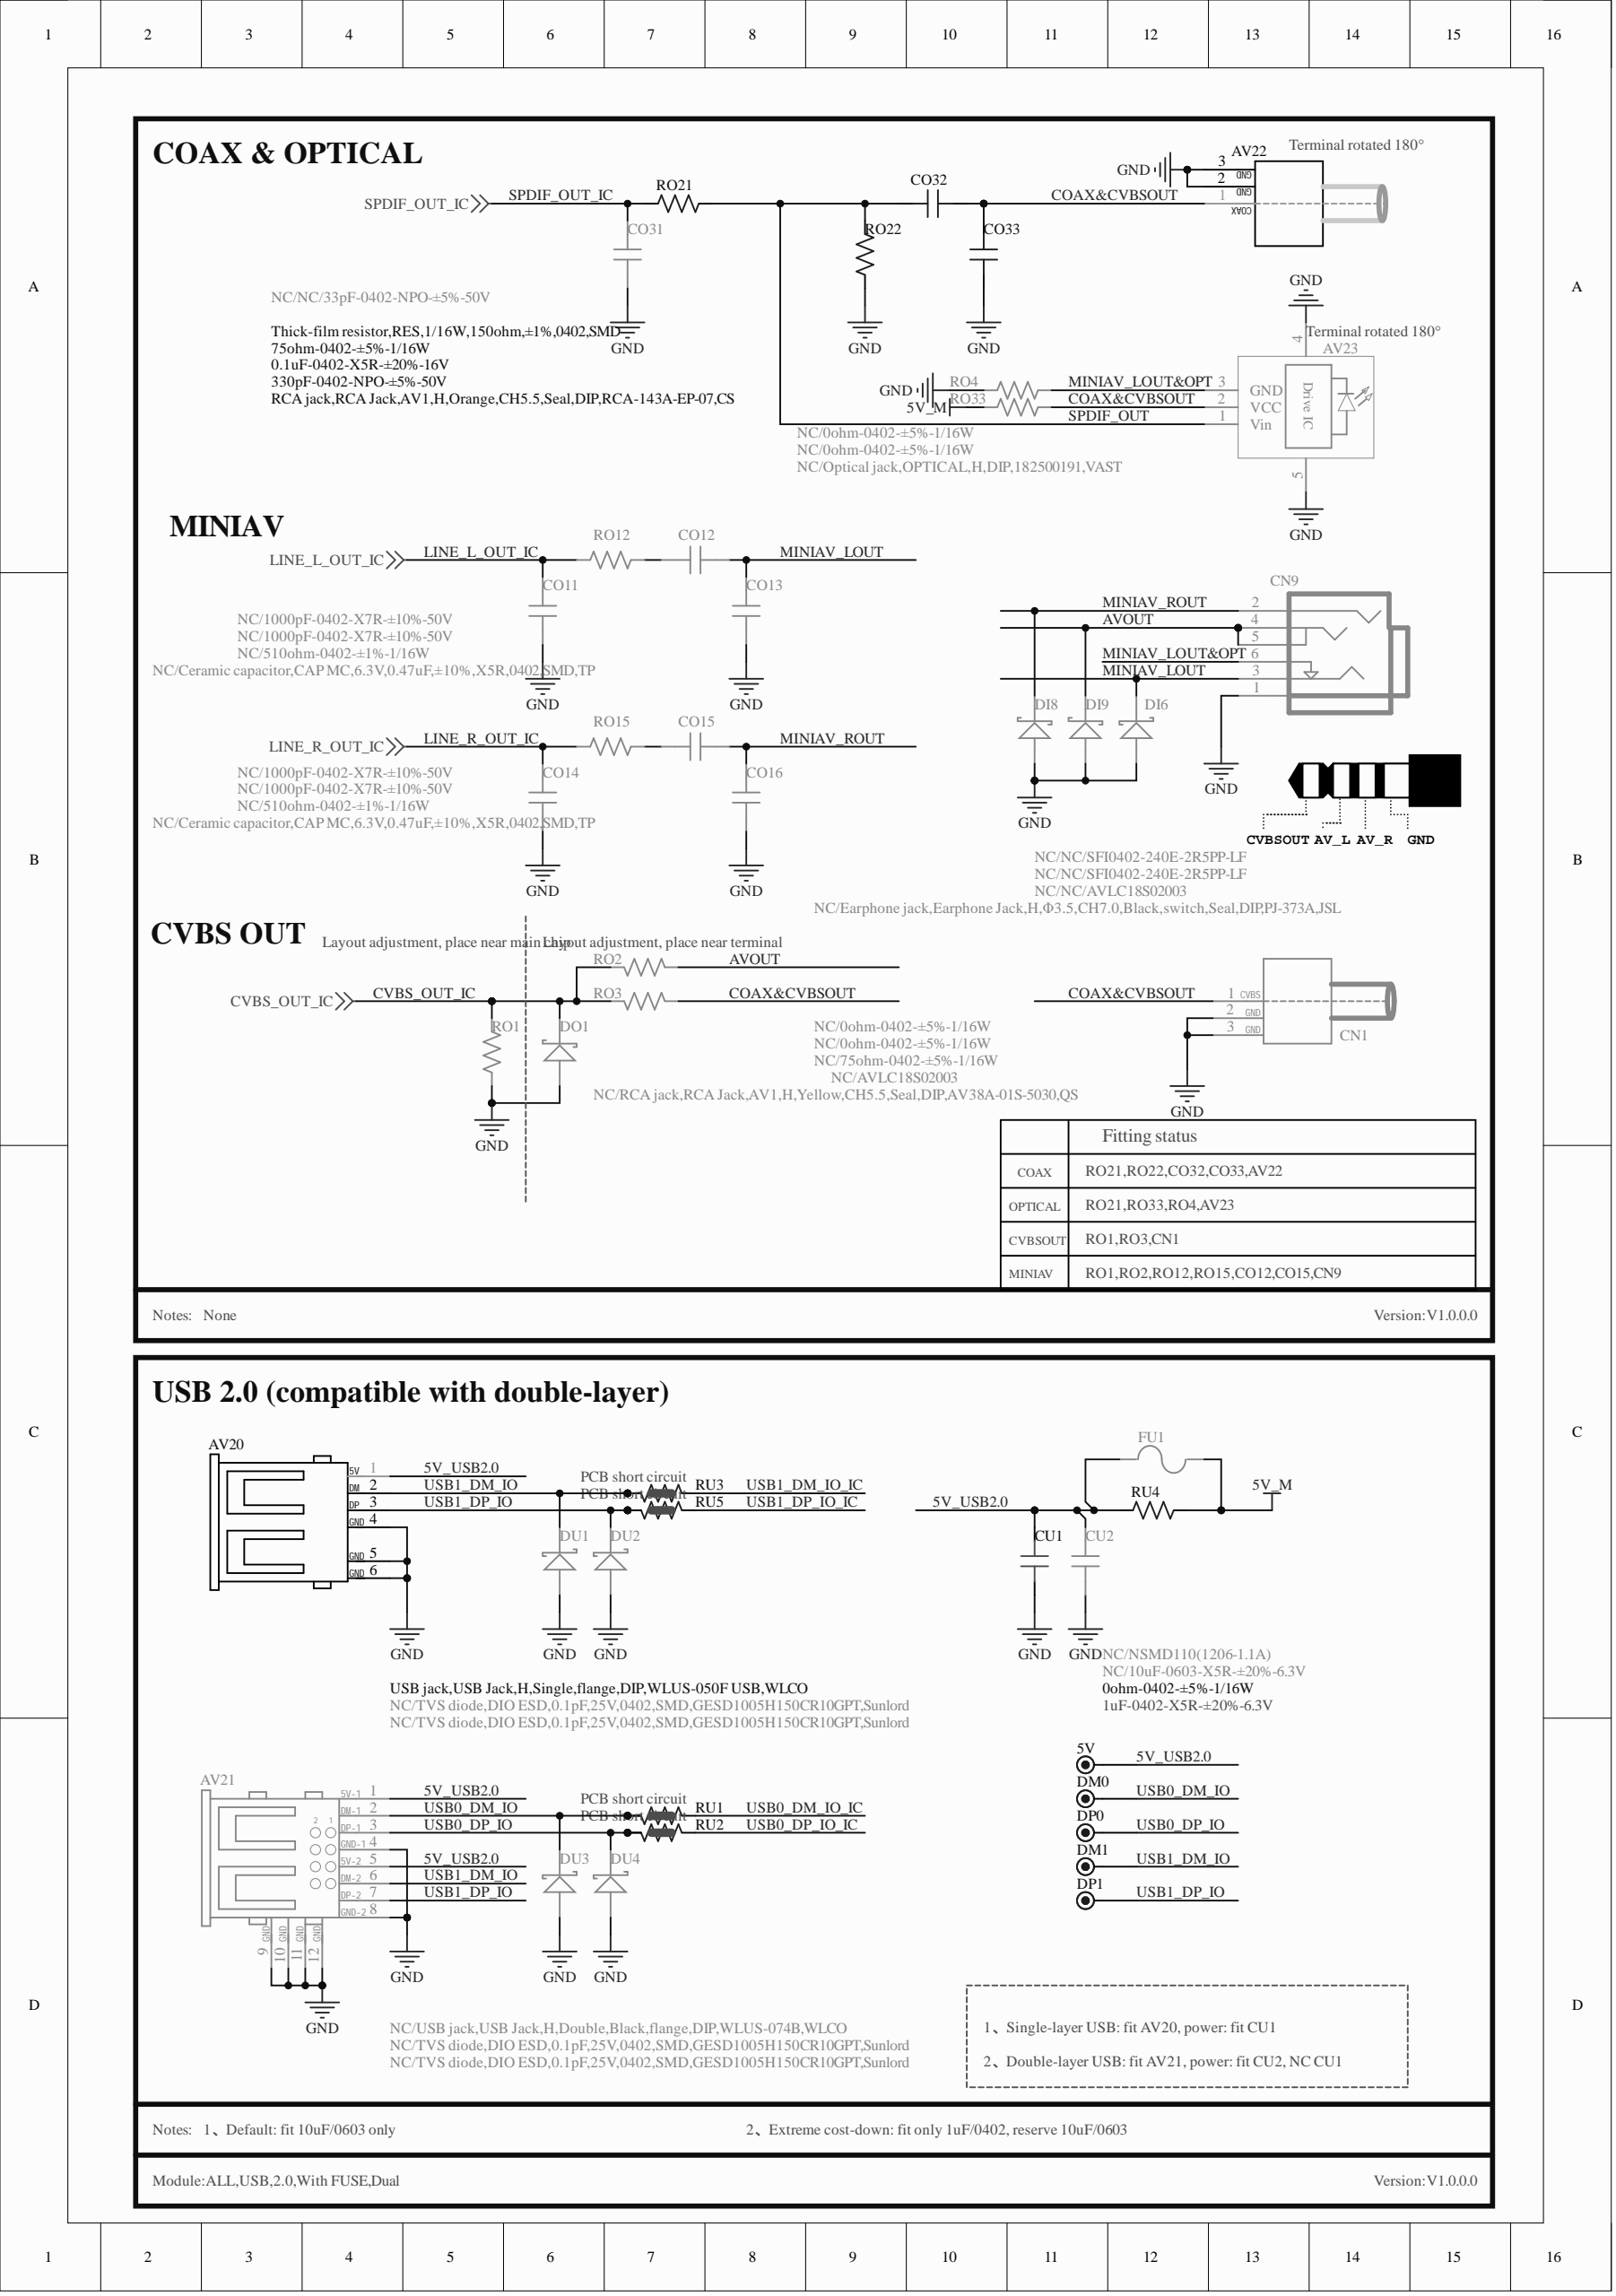Circuit board | Altium Designer | 578 parts | 300 nets | one sheet of the schematic
Parts on this sheet (reference | value | footprint):
5V | DM0 | TP
AV20 | USB jack,USB Jack,H,Single,flange,DIP,WLUS-050F USB,WLCO | USB1-HD-2
AV21 | NC/USB jack,USB Jack,H,Double,Black,flange,DIP,WLUS-074B,WLCO | USB2-HD-1
AV22 | RCA jack,RCA Jack,AV1,H,Orange,CH5.5,Seal,DIP,RCA-143A-EP-07,CS | AV1-H-4
AV23 | NC/Optical jack,OPTICAL,H,DIP,182500191,VAST | OPTICAL-HD-3
CN1 | NC/RCA jack,RCA Jack,AV1,H,Yellow,CH5.5,Seal,DIP,AV38A-01S-5030,QS | AV1-H-4
CN9 | NC/Earphone jack,Earphone Jack,H,F3.5,CH7.0,Black,switch,Seal,DIP,PJ-373A,JSL | PHONE-HD-42
CO11 | NC/1000pF-0402-X7R-±10%-50V | C0402
CO12 | NC/Ceramic capacitor,CAP MC,6.3V,0.47uF,±10%,X5R,0402,SMD,TP | C0402
CO13 | NC/1000pF-0402-X7R-±10%-50V | C0402
CO14 | NC/1000pF-0402-X7R-±10%-50V | C0402
CO15 | NC/Ceramic capacitor,CAP MC,6.3V,0.47uF,±10%,X5R,0402,SMD,TP | C0402
CO16 | NC/1000pF-0402-X7R-±10%-50V | C0402
CO31 | NC/NC/33pF-0402-NPO-±5%-50V | C0402
CO32 | 0.1uF-0402-X5R-±20%-16V | C0402
CO33 | 330pF-0402-NPO-±5%-50V | C0402
CU1 | 1uF-0402-X5R-±20%-6.3V | C0402
CU2 | NC/10uF-0603-X5R-±20%-6.3V | C0603
DI6 | NC/NC/AVLC18S02003 | DIODE-S0402
DI8 | NC/NC/SFI0402-240E-2R5PP-LF | DIODE-S0402
DI9 | NC/NC/SFI0402-240E-2R5PP-LF | DIODE-S0402
DM0 | DM0 | TP
DM1 | DM0 | TP
DO1 | NC/AVLC18S02003 | DIODE-S0402
DP0 | DM0 | TP
DP1 | DM0 | TP
DU1 | NC/TVS diode,DIO ESD,0.1pF,25V,0402,SMD,GESD1005H150CR10GPT,Sunlord | DIODE-S0402
DU2 | NC/TVS diode,DIO ESD,0.1pF,25V,0402,SMD,GESD1005H150CR10GPT,Sunlord | DIODE-S0402
DU3 | NC/TVS diode,DIO ESD,0.1pF,25V,0402,SMD,GESD1005H150CR10GPT,Sunlord | DIODE-S0402
DU4 | NC/TVS diode,DIO ESD,0.1pF,25V,0402,SMD,GESD1005H150CR10GPT,Sunlord | DIODE-S0402
FU1 | NC/NSMD110(1206-1.1A) | FUSE1.1A-S
RO1 | NC/75ohm-0402-±5%-1/16W | R0402
RO2 | NC/0ohm-0402-±5%-1/16W | R0402
RO3 | NC/0ohm-0402-±5%-1/16W | R0402
RO4 | NC/0ohm-0402-±5%-1/16W | R0402
RO12 | NC/510ohm-0402-±1%-1/16W | R0402
RO15 | NC/510ohm-0402-±1%-1/16W | R0402
RO21 | Thick-film resistor,RES,1/16W,150ohm,±1%,0402,SMD | R0402
RO22 | 75ohm-0402-±5%-1/16W | R0402
RO33 | NC/0ohm-0402-±5%-1/16W | R0402
RU1 | NC/0ohm-0402-PCB | R0402SC
RU2 | NC/0ohm-0402-PCB | R0402SC
RU3 | NC/0ohm-0402-PCB | R0402SC
RU4 | 0ohm-0402-±5%-1/16W | R0402
RU5 | NC/0ohm-0402-PCB | R0402SC
Nets of these parts (net: part-pin ...):
USB1_DP_IO_IC: RU5-1
USB1_DP_IO: AV20-3 AV21-7 DP1-1 DU2-K RU5-2 RU5-3
USB1_DM_IO_IC: RU3-1
USB1_DM_IO: AV20-2 AV21-6 DM1-1 DU1-K RU3-2 RU3-3
USB0_DP_IO_IC: RU2-1
USB0_DP_IO: AV21-3 DP0-1 DU4-K RU2-2 RU2-3
USB0_DM_IO_IC: RU1-1
USB0_DM_IO: AV21-2 DM0-1 DU3-K RU1-2 RU1-3
SPDIF_OUT_IC: CO31-2 RO21-1
SPDIF_OUT: AV23-1 CO32-2 RO21-2 RO22-2
NetCO15_2: CO15-2 RO15-1
NetCO12_2: CO12-2 RO12-1
MINIAV_ROUT: CN9-2 CO15-1 CO16-2 DI8-K
MINIAV_LOUT&OPT: AV23-3 CN9-6 RO4-2
MINIAV_LOUT: CN9-3 CO12-1 CO13-2 DI6-K
LINE_R_OUT_IC: CO14-2 RO15-2
LINE_L_OUT_IC: CO11-2 RO12-2
GND: AV20-4 AV20-5 AV20-6 AV21-4 AV21-8 AV21-9 AV21-10 AV21-11 AV21-12 AV22-2 AV22-3 AV23-4 AV23-5 CN1-2 CN1-3 CN9-1 CO11-1 CO13-1 CO14-1 CO16-1 CO31-1 CO33-1 CU1-2 CU2-2 DI6-A DI8-A DI9-A DO1-A DU1-A DU2-A DU3-A DU4-A RO1-1 RO4-1 RO22-1
CVBS_OUT_IC: DO1-K RO1-2 RO2-2 RO3-2
COAX&CVBSOUT: AV22-1 AV23-2 CN1-1 CO32-1 CO33-2 RO3-1 RO33-2
AVOUT: CN9-4 CN9-5 DI9-K RO2-1
5V_USB2.0: 5V-1 AV20-1 AV21-1 AV21-5 CU1-1 CU2-1 FU1-1 RU4-1
5V_M: FU1-2 RO33-1 RU4-2